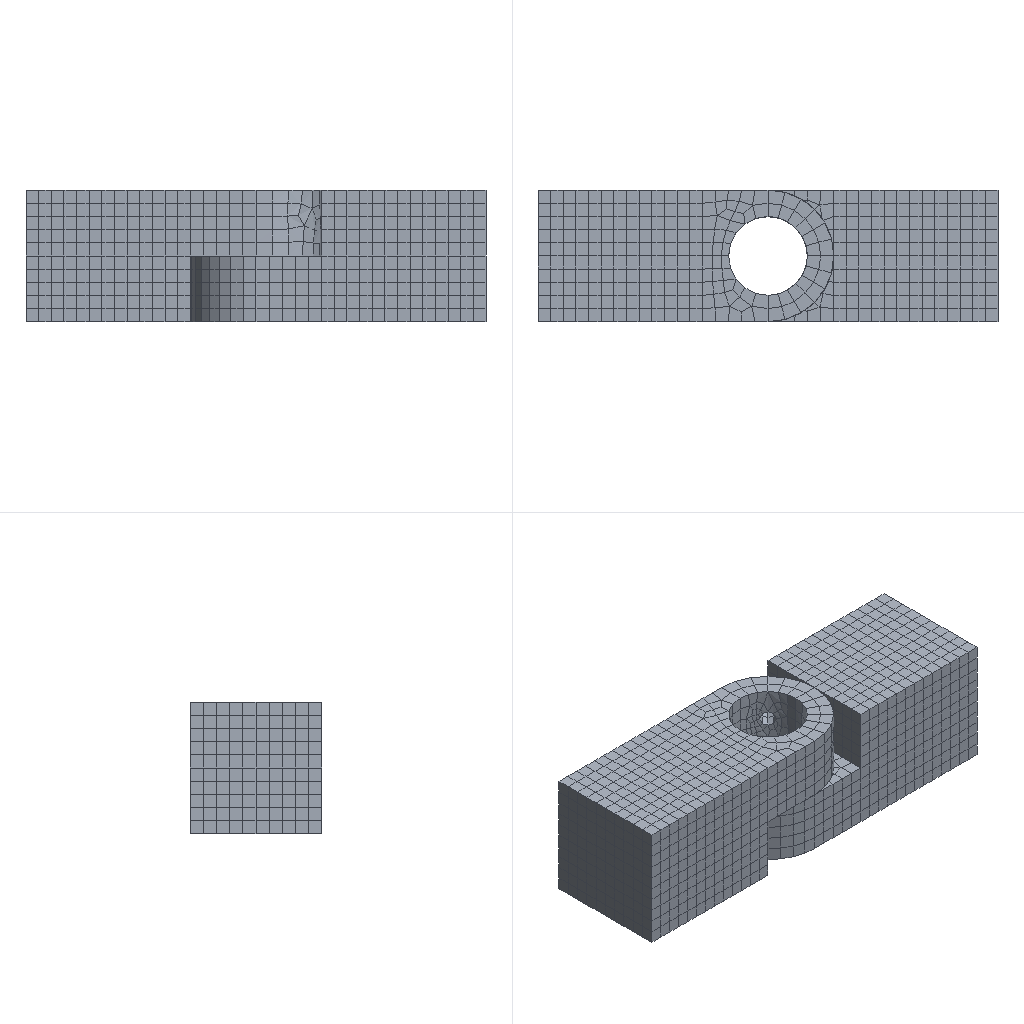Simulation study | abaqus
Set-up summary:
category,name,step,type,value,unit,region
solver,abaqus,,Abaqus/CAE 2024
units,mm-mN-s-kg (kPa) or mm-kg-s,,inferred,E=2e+09 density=
analysis,Contact,,static,time_period=1
analysis,Load,,static,time_period=1
mesh,nodes,,,4526
mesh,elements,,,3364
element_type,C3D8R,,,3364
material,Steel,,E,2e+09
material,Steel,,nu,0.3
section,Steel,,solid section,,,_PickedSet7
section,Steel,,solid section,,,_PickedSet7
load,Pressure,Load,pressure,-10000,,_PickedSurf69
bc,Constrain,initial,fixed,"[dofs=rx,ry,rz,x,y,z n=6]",,Monitor
bc,Fixed,initial,encastre,[dofs=ENCASTRE],,fixed-face-output
bc,NoSlip,initial,fixed,"[dofs=rx,ry,rz,x,y,z n=6]",,_PickedSet68
bc,Constrain,Load,fixed,"[dofs=rx,ry,rz,y,z n=5]",,Monitor
bc,Fixed,Load,encastre,[dofs=ENCASTRE],,fixed-face-output
bc,NoSlip,Load,fixed,"[dofs=rx,rz,y,z n=4]",,_PickedSet68
contact,Flanges,initial,contact pair surface to surface,interaction=NoFric; friction=0; behavior=hard,,Flange-s / Flange-h
contact,Hingein-hole,initial,contact pair surface to surface,interaction=NoFric; friction=0; behavior=hard,,Inside-h / Pin-1.Pin
contact,Hingein-solid,initial,contact pair surface to surface,interaction=NoFric; friction=0; behavior=hard,,Inside-s / Pin-1.Pin
constraint,rigid body,,,1
Abaqus input file, long lists of numbers shortened:
*Heading
** Job name: deck Model name: Model-1
** Generated by: Abaqus/CAE 2024
*Preprint, echo=NO, model=NO, history=NO, contact=NO
**
** PARTS
**
*Part, name=Hinge
*End Part
**
*Part, name=Hinge-solid
*End Part
**
*Part, name=Pin
*End Part
**
**
** ASSEMBLY
**
*Assembly, name=Assembly
**
*Instance, name=Hinge-1, part=Hinge
*Node
      1, -0.025, -0.02, 0.04
      2, -0.025, 0.02, 0.04
** (2265 more lines like these left out)
*Element, type=C3D8R
   1,  124,  629, 1127,  413,    1,   22,  260,   57
   2,  629,  630, 1128, 1127,   22,   23,  261,  260
** (1677 more lines like these left out)
*Nset, nset=_PickedSet7, internal, generate
    1,  2267,     1
*Elset, elset=_PickedSet7, internal, generate
    1,  1679,     1
** Section: Section
*Solid Section, elset=_PickedSet7, material=Steel
1.,
*End Instance
**
*Instance, name=Hinge-solid-1, part=Hinge-solid
        0.09, 1.38777878078145e-17,         0.04
        0.09, 1.38777878078145e-17,         0.04, 0.09,           1.,         0.04,         180.
*Node
      1, -0.025, -0.02, 0.04
      2, -0.025, 0.02, 0.04
** (2256 more lines like these left out)
*Element, type=C3D8R
   1,  119,  605, 1091,  389,    1,   17,  236,   52
   2,  605,  606, 1092, 1091,   17,   18,  237,  236
** (1683 more lines like these left out)
*Nset, nset=_PickedSet7, internal, generate
    1,  2258,     1
*Elset, elset=_PickedSet7, internal, generate
    1,  1685,     1
** Section: Section
*Solid Section, elset=_PickedSet7, material=Steel
1.,
*End Instance
**
*Instance, name=Pin-1, part=Pin
       0.045,           0.,         0.02
       0.045,           0.,         0.02, -0.955,           0.,         0.02, 90.
*Node
      1, 0.012, 0.03,           0.
*Nset, nset=Pin-1-RefPt_, internal
1,
*Surface, type=REVOLUTION, name=Pin
START,        0.012,         0.03
 LINE,        0.012,        -0.03
*Rigid Body, ref node=Pin-1-RefPt_, analytical surface=Pin
*End Instance
**
*Nset, nset=Monitor, instance=Hinge-solid-1
  3,  6, 10, 14, 16
*Nset, nset=Set-output_nodes, instance=Hinge-solid-1
 10,
*Nset, nset=fixed-face-output, instance=Hinge-1
   1,   2,   3,   4,  22,  23,  24,  25,  26,  27,  28,  29,  30,  31,  32,  33
  34,  35,  36,  37,  38,  39,  40,  41,  42,  43,  44,  45,  46,  47,  48,  49
** (6 more lines like these left out)
*Elset, elset=fixed-face-output, instance=Hinge-1, generate
   1,  100,    1
*Nset, nset=hole-output, instance=Hinge-1
  21, 231, 232, 233, 234, 235, 236, 237
*Elset, elset=hole-output, instance=Hinge-1
 1606, 1607, 1613, 1629, 1639, 1645, 1647, 1673
*Nset, nset=_PickedSet68, internal, instance=Pin-1
 1,
*Elset, elset=_Flange-h_S1, internal, instance=Hinge-1, generate
 1301,  1343,     1
*Elset, elset=_Flange-h_S3, internal, instance=Hinge-1
 1517, 1571, 1599, 1653
*Elset, elset=_Flange-h_S6, internal, instance=Hinge-1
 1518, 1543, 1544, 1569, 1600, 1625, 1626, 1651
*Elset, elset=_Flange-h_S4, internal, instance=Hinge-1
 1542, 1567, 1568, 1624, 1649, 1650
*Elset, elset=_Flange-h_S5, internal, instance=Hinge-1
 1545, 1566, 1572, 1627, 1648, 1654
*Surface, type=ELEMENT, name=Flange-h
_Flange-h_S1, S1
_Flange-h_S3, S3
_Flange-h_S6, S6
_Flange-h_S4, S4
_Flange-h_S5, S5
*Elset, elset=_Flange-s_S2, internal, instance=Hinge-solid-1, generate
 1609,  1685,     1
*Surface, type=ELEMENT, name=Flange-s
_Flange-s_S2, S2
*Elset, elset=_Inside-h_S2, internal, instance=Hinge-1, generate
 1598,  1679,     1
*Elset, elset=_Inside-h_S6, internal, instance=Hinge-1
 1301, 1303, 1307, 1313, 1329, 1344, 1346, 1350, 1356, 1372, 1387, 1389, 1393, 1399, 1415, 1430
 1432, 1436, 1442, 1458, 1473, 1475, 1479, 1485, 1501
*Elset, elset=_Inside-h_S3, internal, instance=Hinge-1, generate
 1309,  1481,    43
*Elset, elset=_Inside-h_S4, internal, instance=Hinge-1
 1331, 1333, 1334, 1374, 1376, 1377, 1417, 1419, 1420, 1460, 1462, 1463, 1503, 1505, 1506
*Elset, elset=_Inside-h_S5, internal, instance=Hinge-1, generate
 1335,  1507,    43
*Surface, type=ELEMENT, name=Inside-h
_Inside-h_S2, S2
_Inside-h_S6, S6
_Inside-h_S4, S4
_Inside-h_S3, S3
_Inside-h_S5, S5
*Elset, elset=_Inside-s_S5, internal, instance=Hinge-solid-1
 1307, 1313, 1315, 1341, 1357, 1364, 1384, 1390, 1392, 1418, 1434, 1441, 1461, 1467, 1469, 1495
 1511, 1518, 1538, 1544, 1546, 1572, 1588, 1595, 1615, 1621, 1623, 1649, 1665, 1672
*Elset, elset=_Inside-s_S4, internal, instance=Hinge-solid-1
 1310, 1354, 1387, 1431, 1464, 1508, 1541, 1585, 1618, 1662
*Elset, elset=_Inside-s_S6, internal, instance=Hinge-solid-1
 1312, 1319, 1324, 1325, 1345, 1350, 1356, 1362, 1373, 1389, 1396, 1401, 1402, 1422, 1427, 1433
 1439, 1450, 1466, 1473, 1478, 1479, 1499, 1504, 1510, 1516, 1527, 1543, 1550, 1555, 1556, 1576
** (1 more lines like these left out)
*Elset, elset=_Inside-s_S3, internal, instance=Hinge-solid-1
 1334, 1343, 1346, 1411, 1420, 1423, 1488, 1497, 1500, 1565, 1574, 1577, 1642, 1651, 1654
*Surface, type=ELEMENT, name=Inside-s
_Inside-s_S5, S5
_Inside-s_S4, S4
_Inside-s_S6, S6
_Inside-s_S3, S3
*Elset, elset=__PickedSurf69_S2, internal, instance=Hinge-solid-1, generate
   1,  100,    1
*Surface, type=ELEMENT, name=_PickedSurf69, internal
__PickedSurf69_S2, S2
*End Assembly
**
** MATERIALS
**
*Material, name=Steel
*Elastic
 2e+09, 0.3
**
** INTERACTION PROPERTIES
**
*Surface Interaction, name=NoFric
1.,
*Friction
0.,
*Surface Behavior, pressure-overclosure=HARD
**
** BOUNDARY CONDITIONS
**
** Name: Constrain Type: Displacement/Rotation
*Boundary
Monitor, 1, 1
Monitor, 2, 2
Monitor, 3, 3
Monitor, 4, 4
Monitor, 5, 5
Monitor, 6, 6
** Name: Fixed Type: Symmetry/Antisymmetry/Encastre
*Boundary
fixed-face-output, ENCASTRE
** Name: NoSlip Type: Displacement/Rotation
*Boundary
_PickedSet68, 1, 1
_PickedSet68, 2, 2
_PickedSet68, 3, 3
_PickedSet68, 4, 4
_PickedSet68, 5, 5
_PickedSet68, 6, 6
**
** INTERACTIONS
**
** Interaction: Flanges
*Contact Pair, interaction=NoFric, type=SURFACE TO SURFACE
Flange-s, Flange-h
** Interaction: Hingein-hole
*Contact Pair, interaction=NoFric, type=SURFACE TO SURFACE
Inside-h, Pin-1.Pin
** Interaction: Hingein-solid
*Contact Pair, interaction=NoFric, type=SURFACE TO SURFACE
Inside-s, Pin-1.Pin
** ----------------------------------------------------------------
**
** STEP: Contact
**
*Step, name=Contact, nlgeom=NO
*Static
0.1, 1., 1e-05, 0.1
**
** OUTPUT REQUESTS
**
*Restart, write, frequency=0
*Print, solve=NO
*Monitor, dof=1, node=Set-output_nodes, frequency=1
**
** FIELD OUTPUT: F-Output-1
**
*Output, field
*Node Output
U,
*Element Output, directions=YES
LE, S
*Contact Output
CDISP, CSTRESS
**
** HISTORY OUTPUT: Fixed-face-output
**
*Output, history
*Node Output, nset=fixed-face-output
RF1,
**
** HISTORY OUTPUT: Hole-output
**
*Element Output, elset=hole-output
E11, MISES, S11
**
** HISTORY OUTPUT: H-Output-1
**
*Output, history, frequency=99999
*Node Output, nset=Set-output_nodes
U1, U2, U3
*End Step
** ----------------------------------------------------------------
**
** STEP: Load
**
*Step, name=Load, nlgeom=NO
*Static
0.1, 1., 1e-05, 1.
**
** BOUNDARY CONDITIONS
**
** Name: Constrain Type: Displacement/Rotation
*Boundary, op=NEW
Monitor, 2, 2
Monitor, 3, 3
Monitor, 4, 4
Monitor, 5, 5
Monitor, 6, 6
** Name: Fixed Type: Symmetry/Antisymmetry/Encastre
*Boundary, op=NEW
fixed-face-output, ENCASTRE
** Name: NoSlip Type: Displacement/Rotation
*Boundary, op=NEW
_PickedSet68, 2, 2
_PickedSet68, 3, 3
_PickedSet68, 4, 4
_PickedSet68, 6, 6
**
** LOADS
**
** Name: Pressure   Type: Pressure
*Dsload
_PickedSurf69, P, -10000.
**
** OUTPUT REQUESTS
**
*Restart, write, frequency=0
**
** FIELD OUTPUT: F-Output-1
**
*Output, field
*Node Output
U,
*Element Output, directions=YES
LE, S
*Contact Output
CDISP, CSTRESS
**
** HISTORY OUTPUT: Fixed-face-output
**
*Output, history
*Node Output, nset=fixed-face-output
RF1,
**
** HISTORY OUTPUT: Hole-output
**
*Element Output, elset=hole-output
E11, MISES, S11
**
** HISTORY OUTPUT: H-Output-1
**
*Output, history, frequency=99999
*Node Output, nset=Set-output_nodes
U1, U2, U3
*End Step
Results summary:
result,odb.job_status,,,JOB_STATUS_COMPLETED_SUCCESSFULLY,"consistent, unstated (Abaqus has no unit system)"
result,steps[0].procedure,Contact,,*STATIC,"consistent, unstated (Abaqus has no unit system)"
result,steps[0].time_period,Contact,,1,"consistent, unstated (Abaqus has no unit system)"
result,steps[0].n_frames,Contact,,11,"consistent, unstated (Abaqus has no unit system)"
result,steps[0].last_frame.id,Contact,,10,"consistent, unstated (Abaqus has no unit system)"
result,steps[0].last_frame.value,Contact,,1,"consistent, unstated (Abaqus has no unit system)"
result,steps[0].last_frame.description,Contact,,Increment     10: Step Time =    1.000,"consistent, unstated (Abaqus has no unit system)"
result,steps[0].completed,Contact,,True,"consistent, unstated (Abaqus has no unit system)"
result,steps[0].max_U_magnitude,Contact,,0.0001919,"consistent, unstated (Abaqus has no unit system)"
result,steps[0].max_S_mises,Contact,,1.97477e+07,"consistent, unstated (Abaqus has no unit system)"
result,steps[0].diagnostic.n_increments,Contact,,10,"consistent, unstated (Abaqus has no unit system)"
result,steps[1].procedure,Load,,*STATIC,"consistent, unstated (Abaqus has no unit system)"
result,steps[1].time_period,Load,,1,"consistent, unstated (Abaqus has no unit system)"
result,steps[1].n_frames,Load,,7,"consistent, unstated (Abaqus has no unit system)"
result,steps[1].last_frame.id,Load,,6,"consistent, unstated (Abaqus has no unit system)"
result,steps[1].last_frame.value,Load,,1,"consistent, unstated (Abaqus has no unit system)"
result,steps[1].last_frame.description,Load,,Increment      6: Step Time =    1.000,"consistent, unstated (Abaqus has no unit system)"
result,steps[1].completed,Load,,True,"consistent, unstated (Abaqus has no unit system)"
result,steps[1].max_U_magnitude,Load,,0.0002141,"consistent, unstated (Abaqus has no unit system)"
result,steps[1].max_S_mises,Load,,1.86111e+07,"consistent, unstated (Abaqus has no unit system)"
result,steps[1].diagnostic.n_increments,Load,,6,"consistent, unstated (Abaqus has no unit system)"